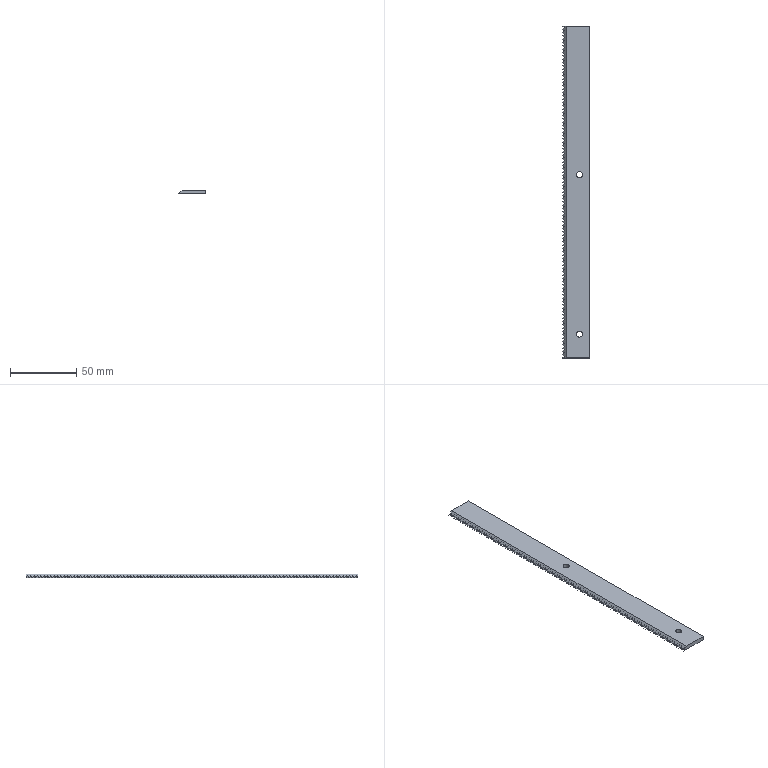Part | SolidWorks | features ICE 2, Chamfer 1, Cut 1, Extrusion 1, LPattern 1, MirrorPattern 1 | 1 solid | 509 faces | box 21 x 250 x 3 mm | volume 14340 mm3 | plane 505 | cylinder 4 | commonest cylinder face diameters 4.6 x4